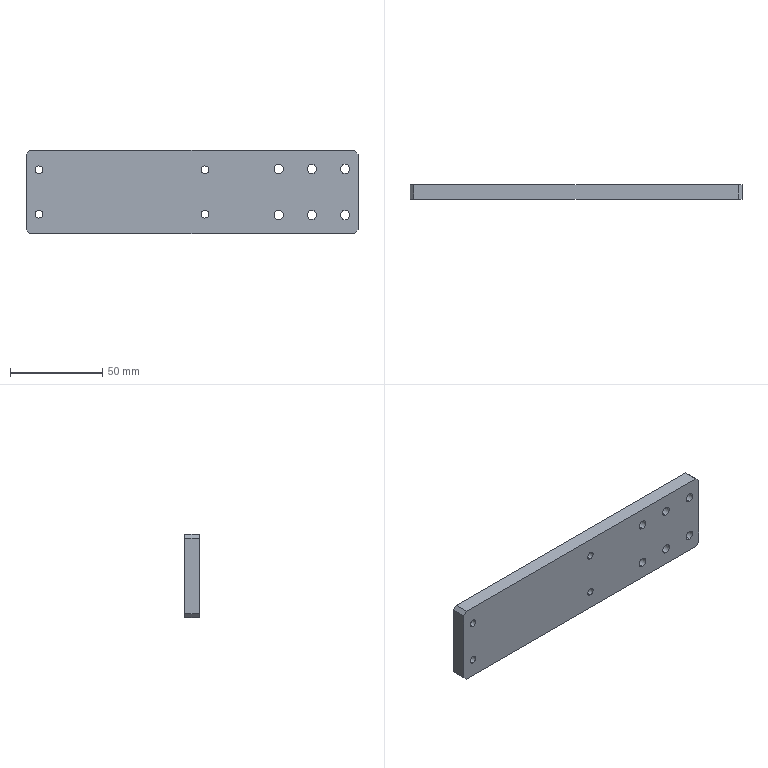Part | STEP file | Cable Carrier Support Plate | 1 solid | 30 faces | box 180 x 8 x 45 mm | volume 63350 mm3 | cylinder 20 | plane 10 | commonest cylinder face diameters 5 x12 4.2 x8